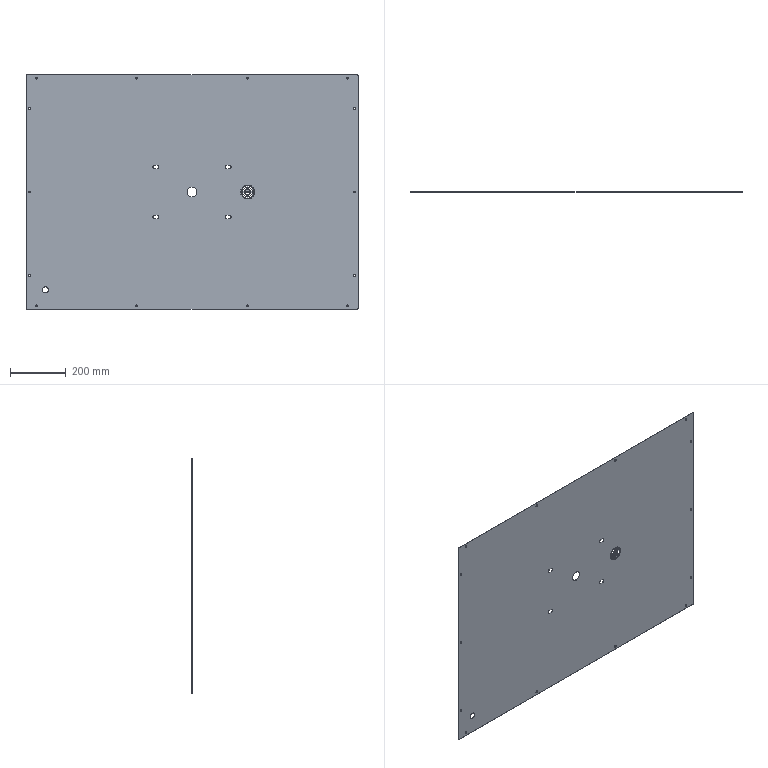Part | SolidWorks | features ICE 5, EdgeFlange 2, HoleWzd 2, Fillet 1, FlatPattern 1, SMBaseFlange 1, SheetMetal 1, WeldmentFeature 1 | 1 solid | 197 faces | box 1195 x 1.2 x 845 mm | volume 1207133 mm3 | cylinder 129 | plane 68 | commonest cylinder face diameters 5.184 x30 6.6 x28 2.074 x26 3.456 x17 1.382 x12 12 x8